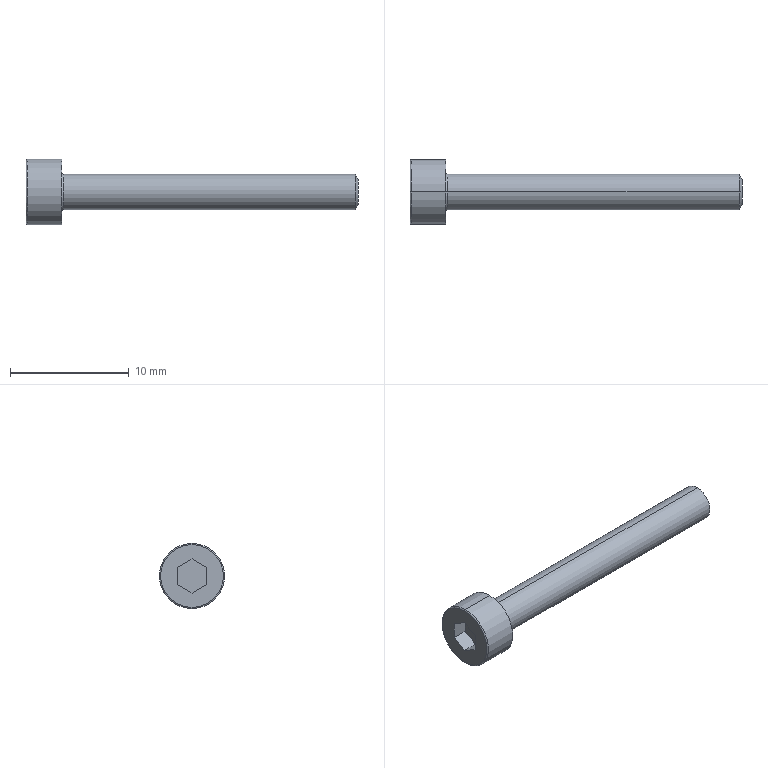Part | STEP file | 1 solid | 20 faces | box 28 x 5.5 x 5.5 mm | volume 240.62 mm3 | plane 10 | torus 4 | cylinder 4 | cone 2 | commonest cylinder face diameters 3 x2 5.5 x2
STEP:
#1=CARTESIAN_POINT('',(0.,0.,2.65));
#2=VERTEX_POINT('',#1);
#3=CARTESIAN_POINT('',(0.,0.,-2.65));
#4=VERTEX_POINT('',#3);
#5=CARTESIAN_POINT('',(0.,0.,0.));
#6=DIRECTION('',(-1.,0.,0.));
#7=DIRECTION('',(0.,0.,-1.));
#8=AXIS2_PLACEMENT_3D('',#5,#6,#7);
#9=CIRCLE('',#8,2.65);
#10=EDGE_CURVE('',#2,#4,#9,.T.);
#11=ORIENTED_EDGE('',*,*,#10,.F.);
#12=CARTESIAN_POINT('',(0.1,0.,2.75));
#13=VERTEX_POINT('',#12);
#14=CARTESIAN_POINT('',(0.1,0.,2.65));
#15=DIRECTION('',(0.,1.,0.));
#16=DIRECTION('',(0.,0.,1.));
#17=AXIS2_PLACEMENT_3D('',#14,#15,#16);
#18=CIRCLE('',#17,0.1);
#19=EDGE_CURVE('',#2,#13,#18,.T.);
#20=ORIENTED_EDGE('',*,*,#19,.T.);
#21=CARTESIAN_POINT('',(0.1,0.,-2.75));
#22=VERTEX_POINT('',#21);
#23=CARTESIAN_POINT('',(0.1,0.,0.));
#24=DIRECTION('',(1.,0.,0.));
#25=DIRECTION('',(0.,0.,-1.));
#26=AXIS2_PLACEMENT_3D('',#23,#24,#25);
#27=CIRCLE('',#26,2.75);
#28=EDGE_CURVE('',#22,#13,#27,.T.);
#29=ORIENTED_EDGE('',*,*,#28,.F.);
#30=CARTESIAN_POINT('',(0.1,0.,-2.65));
#31=DIRECTION('',(0.,-1.,0.));
#32=DIRECTION('',(0.,0.,-1.));
#33=AXIS2_PLACEMENT_3D('',#30,#31,#32);
#34=CIRCLE('',#33,0.1);
#35=EDGE_CURVE('',#4,#22,#34,.T.);
#36=ORIENTED_EDGE('',*,*,#35,.F.);
#37=EDGE_LOOP('',(#11,#20,#29,#36));
#38=FACE_OUTER_BOUND('',#37,.T.);
#39=CARTESIAN_POINT('',(0.1,0.,0.));
#40=DIRECTION('',(1.,0.,0.));
#41=DIRECTION('',(0.,0.,-1.));
#42=AXIS2_PLACEMENT_3D('',#39,#40,#41);
#43=TOROIDAL_SURFACE('',#42,2.65,0.1);
#44=ADVANCED_FACE('',(#38),#43,.T.);
#45=CARTESIAN_POINT('',(28.,0.,1.067));
#46=VERTEX_POINT('',#45);
#47=CARTESIAN_POINT('',(28.,0.,-1.067));
#48=VERTEX_POINT('',#47);
#49=CARTESIAN_POINT('',(28.,0.,0.));
#50=DIRECTION('',(-1.,0.,0.));
#51=DIRECTION('',(0.,0.,1.));
#52=AXIS2_PLACEMENT_3D('',#49,#50,#51);
#53=CIRCLE('',#52,1.067);
#54=EDGE_CURVE('',#46,#48,#53,.T.);
#55=ORIENTED_EDGE('',*,*,#54,.T.);
#56=CARTESIAN_POINT('',(27.75,0.,-1.5));
#57=VERTEX_POINT('',#56);
#58=CARTESIAN_POINT('',(27.75,0.,-1.5));
#59=DIRECTION('',(-0.5,0.,-0.866));
#60=VECTOR('',#59,1000.);
#61=LINE('',#58,#60);
#62=EDGE_CURVE('',#48,#57,#61,.T.);
#63=ORIENTED_EDGE('',*,*,#62,.T.);
#64=CARTESIAN_POINT('',(27.75,0.,1.5));
#65=VERTEX_POINT('',#64);
#66=CARTESIAN_POINT('',(27.75,0.,0.));
#67=DIRECTION('',(-1.,0.,0.));
#68=DIRECTION('',(0.,0.,1.));
#69=AXIS2_PLACEMENT_3D('',#66,#67,#68);
#70=CIRCLE('',#69,1.5);
#71=EDGE_CURVE('',#65,#57,#70,.T.);
#72=ORIENTED_EDGE('',*,*,#71,.F.);
#73=CARTESIAN_POINT('',(27.75,0.,1.5));
#74=DIRECTION('',(-0.5,0.,0.866));
#75=VECTOR('',#74,1000.);
#76=LINE('',#73,#75);
#77=EDGE_CURVE('',#46,#65,#76,.T.);
#78=ORIENTED_EDGE('',*,*,#77,.F.);
#79=EDGE_LOOP('',(#55,#63,#72,#78));
#80=FACE_OUTER_BOUND('',#79,.T.);
#81=CARTESIAN_POINT('',(27.75,0.,0.));
#82=DIRECTION('',(-1.,0.,0.));
#83=DIRECTION('',(0.,0.,1.));
#84=AXIS2_PLACEMENT_3D('',#81,#82,#83);
#85=CONICAL_SURFACE('',#84,1.5,1.047);
#86=ADVANCED_FACE('',(#80),#85,.T.);
#87=CARTESIAN_POINT('',(3.,0.,-1.7));
#88=VERTEX_POINT('',#87);
#89=CARTESIAN_POINT('',(3.,0.,1.7));
#90=VERTEX_POINT('',#89);
#91=CARTESIAN_POINT('',(3.,0.,0.));
#92=DIRECTION('',(-1.,0.,0.));
#93=DIRECTION('',(0.,0.,1.));
#94=AXIS2_PLACEMENT_3D('',#91,#92,#93);
#95=CIRCLE('',#94,1.7);
#96=EDGE_CURVE('',#88,#90,#95,.T.);
#97=ORIENTED_EDGE('',*,*,#96,.F.);
#98=CARTESIAN_POINT('',(3.2,0.,-1.5));
#99=VERTEX_POINT('',#98);
#100=CARTESIAN_POINT('',(3.2,0.,-1.7));
#101=DIRECTION('',(0.,1.,0.));
#102=DIRECTION('',(0.,0.,1.));
#103=AXIS2_PLACEMENT_3D('',#100,#101,#102);
#104=CIRCLE('',#103,0.2);
#105=EDGE_CURVE('',#88,#99,#104,.T.);
#106=ORIENTED_EDGE('',*,*,#105,.T.);
#107=CARTESIAN_POINT('',(3.2,0.,1.5));
#108=VERTEX_POINT('',#107);
#109=CARTESIAN_POINT('',(3.2,0.,0.));
#110=DIRECTION('',(-1.,0.,0.));
#111=DIRECTION('',(0.,0.,1.));
#112=AXIS2_PLACEMENT_3D('',#109,#110,#111);
#113=CIRCLE('',#112,1.5);
#114=EDGE_CURVE('',#99,#108,#113,.T.);
#115=ORIENTED_EDGE('',*,*,#114,.T.);
#116=CARTESIAN_POINT('',(3.2,0.,1.7));
#117=DIRECTION('',(0.,-1.,0.));
#118=DIRECTION('',(0.,0.,-1.));
#119=AXIS2_PLACEMENT_3D('',#116,#117,#118);
#120=CIRCLE('',#119,0.2);
#121=EDGE_CURVE('',#90,#108,#120,.T.);
#122=ORIENTED_EDGE('',*,*,#121,.F.);
#123=EDGE_LOOP('',(#97,#106,#115,#122));
#124=FACE_OUTER_BOUND('',#123,.T.);
#125=CARTESIAN_POINT('',(3.2,0.,0.));
#126=DIRECTION('',(-1.,0.,0.));
#127=DIRECTION('',(0.,0.,1.));
#128=AXIS2_PLACEMENT_3D('',#125,#126,#127);
#129=TOROIDAL_SURFACE('',#128,1.7,0.2);
#130=ADVANCED_FACE('',(#124),#129,.F.);
#131=CARTESIAN_POINT('',(3.,0.,2.75));
#132=VERTEX_POINT('',#131);
#133=CARTESIAN_POINT('',(3.,0.,-2.75));
#134=VERTEX_POINT('',#133);
#135=CARTESIAN_POINT('',(3.,0.,0.));
#136=DIRECTION('',(-1.,0.,0.));
#137=DIRECTION('',(0.,0.,1.));
#138=AXIS2_PLACEMENT_3D('',#135,#136,#137);
#139=CIRCLE('',#138,2.75);
#140=EDGE_CURVE('',#132,#134,#139,.T.);
#141=ORIENTED_EDGE('',*,*,#140,.T.);
#142=CARTESIAN_POINT('',(0.,0.,-2.75));
#143=DIRECTION('',(-1.,0.,0.));
#144=VECTOR('',#143,1000.);
#145=LINE('',#142,#144);
#146=EDGE_CURVE('',#134,#22,#145,.T.);
#147=ORIENTED_EDGE('',*,*,#146,.T.);
#148=ORIENTED_EDGE('',*,*,#28,.T.);
#149=CARTESIAN_POINT('',(0.,0.,2.75));
#150=DIRECTION('',(-1.,0.,0.));
#151=VECTOR('',#150,1000.);
#152=LINE('',#149,#151);
#153=EDGE_CURVE('',#132,#13,#152,.T.);
#154=ORIENTED_EDGE('',*,*,#153,.F.);
#155=EDGE_LOOP('',(#141,#147,#148,#154));
#156=FACE_OUTER_BOUND('',#155,.T.);
#157=CARTESIAN_POINT('',(0.,0.,0.));
#158=DIRECTION('',(-1.,0.,0.));
#159=DIRECTION('',(0.,0.,1.));
#160=AXIS2_PLACEMENT_3D('',#157,#158,#159);
#161=CYLINDRICAL_SURFACE('',#160,2.75);
#162=ADVANCED_FACE('',(#156),#161,.T.);
#163=ORIENTED_EDGE('',*,*,#71,.T.);
#164=CARTESIAN_POINT('',(0.,0.,-1.5));
#165=DIRECTION('',(-1.,0.,0.));
#166=VECTOR('',#165,1000.);
#167=LINE('',#164,#166);
#168=EDGE_CURVE('',#57,#99,#167,.T.);
#169=ORIENTED_EDGE('',*,*,#168,.T.);
#170=CARTESIAN_POINT('',(3.2,0.,0.));
#171=DIRECTION('',(-1.,0.,0.));
#172=DIRECTION('',(0.,0.,1.));
#173=AXIS2_PLACEMENT_3D('',#170,#171,#172);
#174=CIRCLE('',#173,1.5);
#175=EDGE_CURVE('',#108,#99,#174,.T.);
#176=ORIENTED_EDGE('',*,*,#175,.F.);
#177=CARTESIAN_POINT('',(0.,0.,1.5));
#178=DIRECTION('',(-1.,0.,0.));
#179=VECTOR('',#178,1000.);
#180=LINE('',#177,#179);
#181=EDGE_CURVE('',#65,#108,#180,.T.);
#182=ORIENTED_EDGE('',*,*,#181,.F.);
#183=EDGE_LOOP('',(#163,#169,#176,#182));
#184=FACE_OUTER_BOUND('',#183,.T.);
#185=CARTESIAN_POINT('',(0.,0.,0.));
#186=DIRECTION('',(-1.,0.,0.));
#187=DIRECTION('',(0.,0.,1.));
#188=AXIS2_PLACEMENT_3D('',#185,#186,#187);
#189=CYLINDRICAL_SURFACE('',#188,1.5);
#190=ADVANCED_FACE('',(#184),#189,.T.);
#191=ORIENTED_EDGE('',*,*,#168,.F.);
#192=CARTESIAN_POINT('',(27.75,0.,0.));
#193=DIRECTION('',(-1.,0.,0.));
#194=DIRECTION('',(0.,0.,1.));
#195=AXIS2_PLACEMENT_3D('',#192,#193,#194);
#196=CIRCLE('',#195,1.5);
#197=EDGE_CURVE('',#57,#65,#196,.T.);
#198=ORIENTED_EDGE('',*,*,#197,.T.);
#199=ORIENTED_EDGE('',*,*,#181,.T.);
#200=ORIENTED_EDGE('',*,*,#114,.F.);
#201=EDGE_LOOP('',(#191,#198,#199,#200));
#202=FACE_OUTER_BOUND('',#201,.T.);
#203=CARTESIAN_POINT('',(0.,0.,0.));
#204=DIRECTION('',(-1.,0.,0.));
#205=DIRECTION('',(0.,0.,1.));
#206=AXIS2_PLACEMENT_3D('',#203,#204,#205);
#207=CYLINDRICAL_SURFACE('',#206,1.5);
#208=ADVANCED_FACE('',(#202),#207,.T.);
#209=CARTESIAN_POINT('',(0.,0.,0.));
#210=DIRECTION('',(-1.,0.,0.));
#211=DIRECTION('',(0.,0.,-1.));
#212=AXIS2_PLACEMENT_3D('',#209,#210,#211);
#213=CIRCLE('',#212,2.65);
#214=EDGE_CURVE('',#4,#2,#213,.T.);
#215=ORIENTED_EDGE('',*,*,#214,.T.);
#216=ORIENTED_EDGE('',*,*,#10,.T.);
#217=EDGE_LOOP('',(#215,#216));
#218=FACE_OUTER_BOUND('',#217,.T.);
#219=CARTESIAN_POINT('',(0.,0.,1.435));
#220=VERTEX_POINT('',#219);
#221=CARTESIAN_POINT('',(0.,1.243,0.7175));
#222=VERTEX_POINT('',#221);
#223=CARTESIAN_POINT('',(0.,0.,1.435));
#224=DIRECTION('',(0.,0.866,-0.5));
#225=VECTOR('',#224,1000.);
#226=LINE('',#223,#225);
#227=EDGE_CURVE('',#220,#222,#226,.T.);
#228=ORIENTED_EDGE('',*,*,#227,.F.);
#229=CARTESIAN_POINT('',(0.,-1.243,0.7175));
#230=VERTEX_POINT('',#229);
#231=CARTESIAN_POINT('',(0.,-1.243,0.7175));
#232=DIRECTION('',(0.,0.866,0.5));
#233=VECTOR('',#232,1000.);
#234=LINE('',#231,#233);
#235=EDGE_CURVE('',#230,#220,#234,.T.);
#236=ORIENTED_EDGE('',*,*,#235,.F.);
#237=CARTESIAN_POINT('',(0.,-1.243,-0.7175));
#238=VERTEX_POINT('',#237);
#239=CARTESIAN_POINT('',(0.,-1.243,-0.7175));
#240=DIRECTION('',(0.,0.,1.));
#241=VECTOR('',#240,1000.);
#242=LINE('',#239,#241);
#243=EDGE_CURVE('',#238,#230,#242,.T.);
#244=ORIENTED_EDGE('',*,*,#243,.F.);
#245=CARTESIAN_POINT('',(0.,0.,-1.435));
#246=VERTEX_POINT('',#245);
#247=CARTESIAN_POINT('',(0.,0.,-1.435));
#248=DIRECTION('',(0.,-0.866,0.5));
#249=VECTOR('',#248,1000.);
#250=LINE('',#247,#249);
#251=EDGE_CURVE('',#246,#238,#250,.T.);
#252=ORIENTED_EDGE('',*,*,#251,.F.);
#253=CARTESIAN_POINT('',(0.,1.243,-0.7175));
#254=VERTEX_POINT('',#253);
#255=CARTESIAN_POINT('',(0.,1.243,-0.7175));
#256=DIRECTION('',(0.,-0.866,-0.5));
#257=VECTOR('',#256,1000.);
#258=LINE('',#255,#257);
#259=EDGE_CURVE('',#254,#246,#258,.T.);
#260=ORIENTED_EDGE('',*,*,#259,.F.);
#261=CARTESIAN_POINT('',(0.,1.243,0.7175));
#262=DIRECTION('',(0.,0.,-1.));
#263=VECTOR('',#262,1000.);
#264=LINE('',#261,#263);
#265=EDGE_CURVE('',#222,#254,#264,.T.);
#266=ORIENTED_EDGE('',*,*,#265,.F.);
#267=EDGE_LOOP('',(#228,#236,#244,#252,#260,#266));
#268=FACE_BOUND('',#267,.T.);
#269=CARTESIAN_POINT('',(0.,0.,0.));
#270=DIRECTION('',(1.,0.,0.));
#271=DIRECTION('',(0.,0.,-1.));
#272=AXIS2_PLACEMENT_3D('',#269,#270,#271);
#273=PLANE('',#272);
#274=ADVANCED_FACE('',(#218,#268),#273,.F.);
#275=ORIENTED_EDGE('',*,*,#146,.F.);
#276=CARTESIAN_POINT('',(3.,0.,0.));
#277=DIRECTION('',(-1.,0.,0.));
#278=DIRECTION('',(0.,0.,1.));
#279=AXIS2_PLACEMENT_3D('',#276,#277,#278);
#280=CIRCLE('',#279,2.75);
#281=EDGE_CURVE('',#134,#132,#280,.T.);
#282=ORIENTED_EDGE('',*,*,#281,.T.);
#283=ORIENTED_EDGE('',*,*,#153,.T.);
#284=CARTESIAN_POINT('',(0.1,0.,0.));
#285=DIRECTION('',(1.,0.,0.));
#286=DIRECTION('',(0.,0.,-1.));
#287=AXIS2_PLACEMENT_3D('',#284,#285,#286);
#288=CIRCLE('',#287,2.75);
#289=EDGE_CURVE('',#13,#22,#288,.T.);
#290=ORIENTED_EDGE('',*,*,#289,.T.);
#291=EDGE_LOOP('',(#275,#282,#283,#290));
#292=FACE_OUTER_BOUND('',#291,.T.);
#293=CARTESIAN_POINT('',(0.,0.,0.));
#294=DIRECTION('',(-1.,0.,0.));
#295=DIRECTION('',(0.,0.,1.));
#296=AXIS2_PLACEMENT_3D('',#293,#294,#295);
#297=CYLINDRICAL_SURFACE('',#296,2.75);
#298=ADVANCED_FACE('',(#292),#297,.T.);
#299=ORIENTED_EDGE('',*,*,#140,.F.);
#300=ORIENTED_EDGE('',*,*,#281,.F.);
#301=EDGE_LOOP('',(#299,#300));
#302=FACE_OUTER_BOUND('',#301,.T.);
#303=CARTESIAN_POINT('',(3.,0.,0.));
#304=DIRECTION('',(-1.,0.,0.));
#305=DIRECTION('',(0.,0.,1.));
#306=AXIS2_PLACEMENT_3D('',#303,#304,#305);
#307=CIRCLE('',#306,1.7);
#308=EDGE_CURVE('',#90,#88,#307,.T.);
#309=ORIENTED_EDGE('',*,*,#308,.T.);
#310=ORIENTED_EDGE('',*,*,#96,.T.);
#311=EDGE_LOOP('',(#309,#310));
#312=FACE_BOUND('',#311,.T.);
#313=CARTESIAN_POINT('',(3.,2.75,0.));
#314=DIRECTION('',(-1.,0.,0.));
#315=DIRECTION('',(0.,0.,1.));
#316=AXIS2_PLACEMENT_3D('',#313,#314,#315);
#317=PLANE('',#316);
#318=ADVANCED_FACE('',(#302,#312),#317,.F.);
#319=ORIENTED_EDGE('',*,*,#105,.F.);
#320=ORIENTED_EDGE('',*,*,#308,.F.);
#321=ORIENTED_EDGE('',*,*,#121,.T.);
#322=ORIENTED_EDGE('',*,*,#175,.T.);
#323=EDGE_LOOP('',(#319,#320,#321,#322));
#324=FACE_OUTER_BOUND('',#323,.T.);
#325=CARTESIAN_POINT('',(3.2,0.,0.));
#326=DIRECTION('',(-1.,0.,0.));
#327=DIRECTION('',(0.,0.,1.));
#328=AXIS2_PLACEMENT_3D('',#325,#326,#327);
#329=TOROIDAL_SURFACE('',#328,1.7,0.2);
#330=ADVANCED_FACE('',(#324),#329,.F.);
#331=ORIENTED_EDGE('',*,*,#235,.T.);
#332=CARTESIAN_POINT('',(1.3,0.,1.435));
#333=VERTEX_POINT('',#332);
#334=CARTESIAN_POINT('',(1.3,0.,1.435));
#335=DIRECTION('',(-1.,0.,0.));
#336=VECTOR('',#335,1000.);
#337=LINE('',#334,#336);
#338=EDGE_CURVE('',#333,#220,#337,.T.);
#339=ORIENTED_EDGE('',*,*,#338,.F.);
#340=CARTESIAN_POINT('',(1.3,-1.243,0.7175));
#341=VERTEX_POINT('',#340);
#342=CARTESIAN_POINT('',(1.3,-1.243,0.7175));
#343=DIRECTION('',(0.,0.866,0.5));
#344=VECTOR('',#343,1000.);
#345=LINE('',#342,#344);
#346=EDGE_CURVE('',#341,#333,#345,.T.);
#347=ORIENTED_EDGE('',*,*,#346,.F.);
#348=CARTESIAN_POINT('',(1.3,-1.243,0.7175));
#349=DIRECTION('',(-1.,0.,0.));
#350=VECTOR('',#349,1000.);
#351=LINE('',#348,#350);
#352=EDGE_CURVE('',#341,#230,#351,.T.);
#353=ORIENTED_EDGE('',*,*,#352,.T.);
#354=EDGE_LOOP('',(#331,#339,#347,#353));
#355=FACE_OUTER_BOUND('',#354,.T.);
#356=CARTESIAN_POINT('',(1.3,-1.243,0.7175));
#357=DIRECTION('',(0.,-0.5,0.866));
#358=DIRECTION('',(0.,-0.866,-0.5));
#359=AXIS2_PLACEMENT_3D('',#356,#357,#358);
#360=PLANE('',#359);
#361=ADVANCED_FACE('',(#355),#360,.F.);
#362=ORIENTED_EDGE('',*,*,#243,.T.);
#363=ORIENTED_EDGE('',*,*,#352,.F.);
#364=CARTESIAN_POINT('',(1.3,-1.243,-0.7175));
#365=VERTEX_POINT('',#364);
#366=CARTESIAN_POINT('',(1.3,-1.243,-0.7175));
#367=DIRECTION('',(0.,0.,1.));
#368=VECTOR('',#367,1000.);
#369=LINE('',#366,#368);
#370=EDGE_CURVE('',#365,#341,#369,.T.);
#371=ORIENTED_EDGE('',*,*,#370,.F.);
#372=CARTESIAN_POINT('',(1.3,-1.243,-0.7175));
#373=DIRECTION('',(-1.,0.,0.));
#374=VECTOR('',#373,1000.);
#375=LINE('',#372,#374);
#376=EDGE_CURVE('',#365,#238,#375,.T.);
#377=ORIENTED_EDGE('',*,*,#376,.T.);
#378=EDGE_LOOP('',(#362,#363,#371,#377));
#379=FACE_OUTER_BOUND('',#378,.T.);
#380=CARTESIAN_POINT('',(1.3,-1.243,-0.7175));
#381=DIRECTION('',(0.,-1.,0.));
#382=DIRECTION('',(0.,0.,-1.));
#383=AXIS2_PLACEMENT_3D('',#380,#381,#382);
#384=PLANE('',#383);
#385=ADVANCED_FACE('',(#379),#384,.F.);
#386=ORIENTED_EDGE('',*,*,#251,.T.);
#387=ORIENTED_EDGE('',*,*,#376,.F.);
#388=CARTESIAN_POINT('',(1.3,0.,-1.435));
#389=VERTEX_POINT('',#388);
#390=CARTESIAN_POINT('',(1.3,0.,-1.435));
#391=DIRECTION('',(0.,-0.866,0.5));
#392=VECTOR('',#391,1000.);
#393=LINE('',#390,#392);
#394=EDGE_CURVE('',#389,#365,#393,.T.);
#395=ORIENTED_EDGE('',*,*,#394,.F.);
#396=CARTESIAN_POINT('',(1.3,0.,-1.435));
#397=DIRECTION('',(-1.,0.,0.));
#398=VECTOR('',#397,1000.);
#399=LINE('',#396,#398);
#400=EDGE_CURVE('',#389,#246,#399,.T.);
#401=ORIENTED_EDGE('',*,*,#400,.T.);
#402=EDGE_LOOP('',(#386,#387,#395,#401));
#403=FACE_OUTER_BOUND('',#402,.T.);
#404=CARTESIAN_POINT('',(1.3,0.,-1.435));
#405=DIRECTION('',(0.,-0.5,-0.866));
#406=DIRECTION('',(0.,0.866,-0.5));
#407=AXIS2_PLACEMENT_3D('',#404,#405,#406);
#408=PLANE('',#407);
#409=ADVANCED_FACE('',(#403),#408,.F.);
#410=ORIENTED_EDGE('',*,*,#259,.T.);
#411=ORIENTED_EDGE('',*,*,#400,.F.);
#412=CARTESIAN_POINT('',(1.3,1.243,-0.7175));
#413=VERTEX_POINT('',#412);
#414=CARTESIAN_POINT('',(1.3,1.243,-0.7175));
#415=DIRECTION('',(0.,-0.866,-0.5));
#416=VECTOR('',#415,1000.);
#417=LINE('',#414,#416);
#418=EDGE_CURVE('',#413,#389,#417,.T.);
#419=ORIENTED_EDGE('',*,*,#418,.F.);
#420=CARTESIAN_POINT('',(1.3,1.243,-0.7175));
#421=DIRECTION('',(-1.,0.,0.));
#422=VECTOR('',#421,1000.);
#423=LINE('',#420,#422);
#424=EDGE_CURVE('',#413,#254,#423,.T.);
#425=ORIENTED_EDGE('',*,*,#424,.T.);
#426=EDGE_LOOP('',(#410,#411,#419,#425));
#427=FACE_OUTER_BOUND('',#426,.T.);
#428=CARTESIAN_POINT('',(1.3,1.243,-0.7175));
#429=DIRECTION('',(0.,0.5,-0.866));
#430=DIRECTION('',(0.,0.866,0.5));
#431=AXIS2_PLACEMENT_3D('',#428,#429,#430);
#432=PLANE('',#431);
#433=ADVANCED_FACE('',(#427),#432,.F.);
#434=ORIENTED_EDGE('',*,*,#265,.T.);
#435=ORIENTED_EDGE('',*,*,#424,.F.);
#436=CARTESIAN_POINT('',(1.3,1.243,0.7175));
#437=VERTEX_POINT('',#436);
#438=CARTESIAN_POINT('',(1.3,1.243,0.7175));
#439=DIRECTION('',(0.,0.,-1.));
#440=VECTOR('',#439,1000.);
#441=LINE('',#438,#440);
#442=EDGE_CURVE('',#437,#413,#441,.T.);
#443=ORIENTED_EDGE('',*,*,#442,.F.);
#444=CARTESIAN_POINT('',(1.3,1.243,0.7175));
#445=DIRECTION('',(-1.,0.,0.));
#446=VECTOR('',#445,1000.);
#447=LINE('',#444,#446);
#448=EDGE_CURVE('',#437,#222,#447,.T.);
#449=ORIENTED_EDGE('',*,*,#448,.T.);
#450=EDGE_LOOP('',(#434,#435,#443,#449));
#451=FACE_OUTER_BOUND('',#450,.T.);
#452=CARTESIAN_POINT('',(1.3,1.243,0.7175));
#453=DIRECTION('',(0.,1.,0.));
#454=DIRECTION('',(0.,0.,1.));
#455=AXIS2_PLACEMENT_3D('',#452,#453,#454);
#456=PLANE('',#455);
#457=ADVANCED_FACE('',(#451),#456,.F.);
#458=ORIENTED_EDGE('',*,*,#227,.T.);
#459=ORIENTED_EDGE('',*,*,#448,.F.);
#460=CARTESIAN_POINT('',(1.3,0.,1.435));
#461=DIRECTION('',(0.,0.866,-0.5));
#462=VECTOR('',#461,1000.);
#463=LINE('',#460,#462);
#464=EDGE_CURVE('',#333,#437,#463,.T.);
#465=ORIENTED_EDGE('',*,*,#464,.F.);
#466=ORIENTED_EDGE('',*,*,#338,.T.);
#467=EDGE_LOOP('',(#458,#459,#465,#466));
#468=FACE_OUTER_BOUND('',#467,.T.);
#469=CARTESIAN_POINT('',(1.3,0.,1.435));
#470=DIRECTION('',(0.,0.5,0.866));
#471=DIRECTION('',(0.,-0.866,0.5));
#472=AXIS2_PLACEMENT_3D('',#469,#470,#471);
#473=PLANE('',#472);
#474=ADVANCED_FACE('',(#468),#473,.F.);
#475=ORIENTED_EDGE('',*,*,#346,.T.);
#476=ORIENTED_EDGE('',*,*,#464,.T.);
#477=ORIENTED_EDGE('',*,*,#442,.T.);
#478=ORIENTED_EDGE('',*,*,#418,.T.);
#479=ORIENTED_EDGE('',*,*,#394,.T.);
#480=ORIENTED_EDGE('',*,*,#370,.T.);
#481=EDGE_LOOP('',(#475,#476,#477,#478,#479,#480));
#482=FACE_OUTER_BOUND('',#481,.T.);
#483=CARTESIAN_POINT('',(1.3,-1.243,0.7175));
#484=DIRECTION('',(1.,0.,0.));
#485=DIRECTION('',(0.,0.,-1.));
#486=AXIS2_PLACEMENT_3D('',#483,#484,#485);
#487=PLANE('',#486);
#488=ADVANCED_FACE('',(#482),#487,.F.);
#489=ORIENTED_EDGE('',*,*,#62,.F.);
#490=CARTESIAN_POINT('',(28.,0.,0.));
#491=DIRECTION('',(-1.,0.,0.));
#492=DIRECTION('',(0.,0.,1.));
#493=AXIS2_PLACEMENT_3D('',#490,#491,#492);
#494=CIRCLE('',#493,1.067);
#495=EDGE_CURVE('',#48,#46,#494,.T.);
#496=ORIENTED_EDGE('',*,*,#495,.T.);
#497=ORIENTED_EDGE('',*,*,#77,.T.);
#498=ORIENTED_EDGE('',*,*,#197,.F.);
#499=EDGE_LOOP('',(#489,#496,#497,#498));
#500=FACE_OUTER_BOUND('',#499,.T.);
#501=CARTESIAN_POINT('',(27.75,0.,0.));
#502=DIRECTION('',(-1.,0.,0.));
#503=DIRECTION('',(0.,0.,1.));
#504=AXIS2_PLACEMENT_3D('',#501,#502,#503);
#505=CONICAL_SURFACE('',#504,1.5,1.047);
#506=ADVANCED_FACE('',(#500),#505,.T.);
#507=ORIENTED_EDGE('',*,*,#54,.F.);
#508=ORIENTED_EDGE('',*,*,#495,.F.);
#509=EDGE_LOOP('',(#507,#508));
#510=FACE_OUTER_BOUND('',#509,.T.);
#511=CARTESIAN_POINT('',(28.,1.5,0.));
#512=DIRECTION('',(-1.,0.,0.));
#513=DIRECTION('',(0.,0.,1.));
#514=AXIS2_PLACEMENT_3D('',#511,#512,#513);
#515=PLANE('',#514);
#516=ADVANCED_FACE('',(#510),#515,.F.);
#517=ORIENTED_EDGE('',*,*,#19,.F.);
#518=ORIENTED_EDGE('',*,*,#214,.F.);
#519=ORIENTED_EDGE('',*,*,#35,.T.);
#520=ORIENTED_EDGE('',*,*,#289,.F.);
#521=EDGE_LOOP('',(#517,#518,#519,#520));
#522=FACE_OUTER_BOUND('',#521,.T.);
#523=CARTESIAN_POINT('',(0.1,0.,0.));
#524=DIRECTION('',(1.,0.,0.));
#525=DIRECTION('',(0.,0.,-1.));
#526=AXIS2_PLACEMENT_3D('',#523,#524,#525);
#527=TOROIDAL_SURFACE('',#526,2.65,0.1);
#528=ADVANCED_FACE('',(#522),#527,.T.);
#529=CLOSED_SHELL('',(#44,#86,#130,#162,#190,#208,#274,#298,#318,#330,#361,#385,#409,#433,#457,#474,#488,#506,#516,#528));
#530=MANIFOLD_SOLID_BREP('',#529);
#531=CARTESIAN_POINT('',(0.,0.,0.));
#532=DIRECTION('',(0.,0.,1.));
#533=DIRECTION('',(1.,0.,0.));
#534=AXIS2_PLACEMENT_3D('',#531,#532,#533);
#535=(LENGTH_UNIT()NAMED_UNIT(*)SI_UNIT(.MILLI.,.METRE.));
#536=UNCERTAINTY_MEASURE_WITH_UNIT(LENGTH_MEASURE(0.00001),#535,'','');
#537=(NAMED_UNIT(*)PLANE_ANGLE_UNIT()SI_UNIT($,.RADIAN.));
#538=(NAMED_UNIT(*)SI_UNIT($,.STERADIAN.)SOLID_ANGLE_UNIT());
#539=(GEOMETRIC_REPRESENTATION_CONTEXT(3)GLOBAL_UNCERTAINTY_ASSIGNED_CONTEXT((#536))GLOBAL_UNIT_ASSIGNED_CONTEXT((#535,#537,#538))REPRESENTATION_CONTEXT('',''));
#540=ADVANCED_BREP_SHAPE_REPRESENTATION('',(#530,#534),#539);